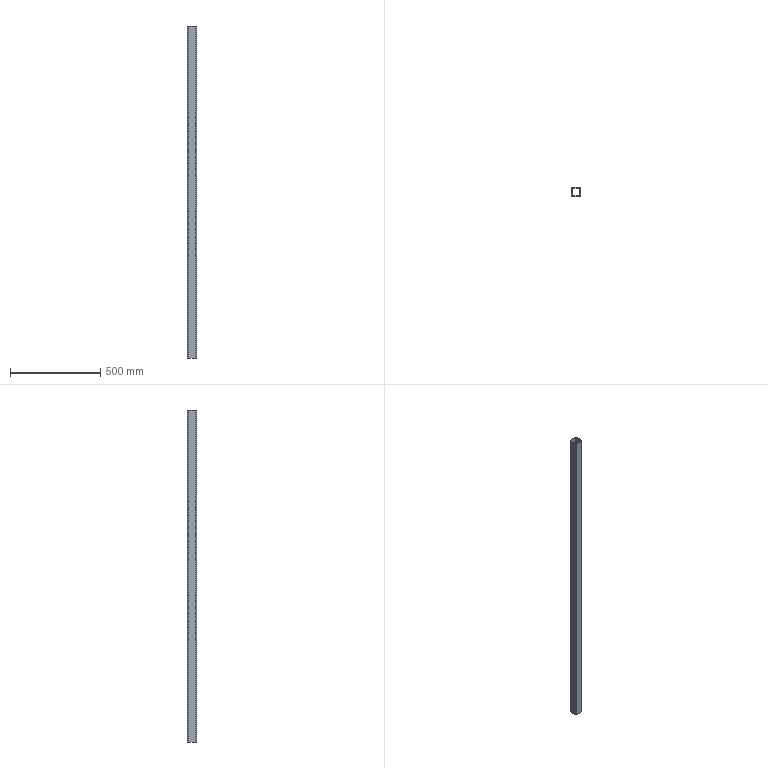Part | SolidWorks | 1 solid | 18 faces | box 50 x 50 x 1840 mm | volume 995114 mm3 | plane 10 | cylinder 8 | commonest cylinder face diameters 6 x4 12 x4
STEP:
#1=CARTESIAN_POINT('',(19.,25.,920.));
#2=VERTEX_POINT('',#1);
#3=CARTESIAN_POINT('',(25.,19.,920.));
#4=VERTEX_POINT('',#3);
#5=CARTESIAN_POINT('',(19.,19.,920.));
#6=DIRECTION('',(0.,0.,-1.));
#7=DIRECTION('',(-1.,0.,0.));
#8=AXIS2_PLACEMENT_3D('',#5,#6,#7);
#9=CIRCLE('',#8,6.);
#10=EDGE_CURVE('',#2,#4,#9,.T.);
#11=ORIENTED_EDGE('',*,*,#10,.T.);
#12=CARTESIAN_POINT('',(25.,19.,-920.));
#13=VERTEX_POINT('',#12);
#14=CARTESIAN_POINT('',(25.,19.,-920.));
#15=DIRECTION('',(0.,0.,1.));
#16=VECTOR('',#15,1000.);
#17=LINE('',#14,#16);
#18=EDGE_CURVE('',#13,#4,#17,.T.);
#19=ORIENTED_EDGE('',*,*,#18,.F.);
#20=CARTESIAN_POINT('',(19.,25.,-920.));
#21=VERTEX_POINT('',#20);
#22=CARTESIAN_POINT('',(19.,19.,-920.));
#23=DIRECTION('',(0.,0.,-1.));
#24=DIRECTION('',(-1.,0.,0.));
#25=AXIS2_PLACEMENT_3D('',#22,#23,#24);
#26=CIRCLE('',#25,6.);
#27=EDGE_CURVE('',#21,#13,#26,.T.);
#28=ORIENTED_EDGE('',*,*,#27,.F.);
#29=CARTESIAN_POINT('',(19.,25.,-920.));
#30=DIRECTION('',(0.,0.,1.));
#31=VECTOR('',#30,1000.);
#32=LINE('',#29,#31);
#33=EDGE_CURVE('',#21,#2,#32,.T.);
#34=ORIENTED_EDGE('',*,*,#33,.T.);
#35=EDGE_LOOP('',(#11,#19,#28,#34));
#36=FACE_OUTER_BOUND('',#35,.T.);
#37=CARTESIAN_POINT('',(19.,19.,-920.));
#38=DIRECTION('',(0.,0.,1.));
#39=DIRECTION('',(1.,0.,0.));
#40=AXIS2_PLACEMENT_3D('',#37,#38,#39);
#41=CYLINDRICAL_SURFACE('',#40,6.);
#42=ADVANCED_FACE('',(#36),#41,.T.);
#43=CARTESIAN_POINT('',(25.,-19.,920.));
#44=VERTEX_POINT('',#43);
#45=CARTESIAN_POINT('',(25.,19.,920.));
#46=DIRECTION('',(0.,-1.,0.));
#47=VECTOR('',#46,1000.);
#48=LINE('',#45,#47);
#49=EDGE_CURVE('',#4,#44,#48,.T.);
#50=ORIENTED_EDGE('',*,*,#49,.T.);
#51=CARTESIAN_POINT('',(25.,-19.,-920.));
#52=VERTEX_POINT('',#51);
#53=CARTESIAN_POINT('',(25.,-19.,-920.));
#54=DIRECTION('',(0.,0.,1.));
#55=VECTOR('',#54,1000.);
#56=LINE('',#53,#55);
#57=EDGE_CURVE('',#52,#44,#56,.T.);
#58=ORIENTED_EDGE('',*,*,#57,.F.);
#59=CARTESIAN_POINT('',(25.,19.,-920.));
#60=DIRECTION('',(0.,-1.,0.));
#61=VECTOR('',#60,1000.);
#62=LINE('',#59,#61);
#63=EDGE_CURVE('',#13,#52,#62,.T.);
#64=ORIENTED_EDGE('',*,*,#63,.F.);
#65=ORIENTED_EDGE('',*,*,#18,.T.);
#66=EDGE_LOOP('',(#50,#58,#64,#65));
#67=FACE_OUTER_BOUND('',#66,.T.);
#68=CARTESIAN_POINT('',(25.,19.,-920.));
#69=DIRECTION('',(-1.,0.,0.));
#70=DIRECTION('',(0.,0.,1.));
#71=AXIS2_PLACEMENT_3D('',#68,#69,#70);
#72=PLANE('',#71);
#73=ADVANCED_FACE('',(#67),#72,.F.);
#74=CARTESIAN_POINT('',(19.,-25.,920.));
#75=VERTEX_POINT('',#74);
#76=CARTESIAN_POINT('',(19.,-19.,920.));
#77=DIRECTION('',(0.,0.,-1.));
#78=DIRECTION('',(-1.,0.,0.));
#79=AXIS2_PLACEMENT_3D('',#76,#77,#78);
#80=CIRCLE('',#79,6.);
#81=EDGE_CURVE('',#44,#75,#80,.T.);
#82=ORIENTED_EDGE('',*,*,#81,.T.);
#83=CARTESIAN_POINT('',(19.,-25.,-920.));
#84=VERTEX_POINT('',#83);
#85=CARTESIAN_POINT('',(19.,-25.,-920.));
#86=DIRECTION('',(0.,0.,1.));
#87=VECTOR('',#86,1000.);
#88=LINE('',#85,#87);
#89=EDGE_CURVE('',#84,#75,#88,.T.);
#90=ORIENTED_EDGE('',*,*,#89,.F.);
#91=CARTESIAN_POINT('',(19.,-19.,-920.));
#92=DIRECTION('',(0.,0.,-1.));
#93=DIRECTION('',(-1.,0.,0.));
#94=AXIS2_PLACEMENT_3D('',#91,#92,#93);
#95=CIRCLE('',#94,6.);
#96=EDGE_CURVE('',#52,#84,#95,.T.);
#97=ORIENTED_EDGE('',*,*,#96,.F.);
#98=ORIENTED_EDGE('',*,*,#57,.T.);
#99=EDGE_LOOP('',(#82,#90,#97,#98));
#100=FACE_OUTER_BOUND('',#99,.T.);
#101=CARTESIAN_POINT('',(19.,-19.,-920.));
#102=DIRECTION('',(0.,0.,1.));
#103=DIRECTION('',(1.,0.,0.));
#104=AXIS2_PLACEMENT_3D('',#101,#102,#103);
#105=CYLINDRICAL_SURFACE('',#104,6.);
#106=ADVANCED_FACE('',(#100),#105,.T.);
#107=CARTESIAN_POINT('',(-19.,-25.,920.));
#108=VERTEX_POINT('',#107);
#109=CARTESIAN_POINT('',(-19.,-25.,920.));
#110=DIRECTION('',(-1.,0.,0.));
#111=VECTOR('',#110,1000.);
#112=LINE('',#109,#111);
#113=EDGE_CURVE('',#75,#108,#112,.T.);
#114=ORIENTED_EDGE('',*,*,#113,.T.);
#115=CARTESIAN_POINT('',(-19.,-25.,-920.));
#116=VERTEX_POINT('',#115);
#117=CARTESIAN_POINT('',(-19.,-25.,-920.));
#118=DIRECTION('',(0.,0.,1.));
#119=VECTOR('',#118,1000.);
#120=LINE('',#117,#119);
#121=EDGE_CURVE('',#116,#108,#120,.T.);
#122=ORIENTED_EDGE('',*,*,#121,.F.);
#123=CARTESIAN_POINT('',(-19.,-25.,-920.));
#124=DIRECTION('',(-1.,0.,0.));
#125=VECTOR('',#124,1000.);
#126=LINE('',#123,#125);
#127=EDGE_CURVE('',#84,#116,#126,.T.);
#128=ORIENTED_EDGE('',*,*,#127,.F.);
#129=ORIENTED_EDGE('',*,*,#89,.T.);
#130=EDGE_LOOP('',(#114,#122,#128,#129));
#131=FACE_OUTER_BOUND('',#130,.T.);
#132=CARTESIAN_POINT('',(-19.,-25.,-920.));
#133=DIRECTION('',(0.,1.,0.));
#134=DIRECTION('',(0.,0.,1.));
#135=AXIS2_PLACEMENT_3D('',#132,#133,#134);
#136=PLANE('',#135);
#137=ADVANCED_FACE('',(#131),#136,.F.);
#138=CARTESIAN_POINT('',(-25.,-19.,920.));
#139=VERTEX_POINT('',#138);
#140=CARTESIAN_POINT('',(-19.,-19.,920.));
#141=DIRECTION('',(0.,0.,-1.));
#142=DIRECTION('',(-1.,0.,0.));
#143=AXIS2_PLACEMENT_3D('',#140,#141,#142);
#144=CIRCLE('',#143,6.);
#145=EDGE_CURVE('',#108,#139,#144,.T.);
#146=ORIENTED_EDGE('',*,*,#145,.T.);
#147=CARTESIAN_POINT('',(-25.,-19.,-920.));
#148=VERTEX_POINT('',#147);
#149=CARTESIAN_POINT('',(-25.,-19.,-920.));
#150=DIRECTION('',(0.,0.,1.));
#151=VECTOR('',#150,1000.);
#152=LINE('',#149,#151);
#153=EDGE_CURVE('',#148,#139,#152,.T.);
#154=ORIENTED_EDGE('',*,*,#153,.F.);
#155=CARTESIAN_POINT('',(-19.,-19.,-920.));
#156=DIRECTION('',(0.,0.,-1.));
#157=DIRECTION('',(-1.,0.,0.));
#158=AXIS2_PLACEMENT_3D('',#155,#156,#157);
#159=CIRCLE('',#158,6.);
#160=EDGE_CURVE('',#116,#148,#159,.T.);
#161=ORIENTED_EDGE('',*,*,#160,.F.);
#162=ORIENTED_EDGE('',*,*,#121,.T.);
#163=EDGE_LOOP('',(#146,#154,#161,#162));
#164=FACE_OUTER_BOUND('',#163,.T.);
#165=CARTESIAN_POINT('',(-19.,-19.,-920.));
#166=DIRECTION('',(0.,0.,1.));
#167=DIRECTION('',(1.,0.,0.));
#168=AXIS2_PLACEMENT_3D('',#165,#166,#167);
#169=CYLINDRICAL_SURFACE('',#168,6.);
#170=ADVANCED_FACE('',(#164),#169,.T.);
#171=CARTESIAN_POINT('',(-25.,19.,920.));
#172=VERTEX_POINT('',#171);
#173=CARTESIAN_POINT('',(-25.,-19.,920.));
#174=DIRECTION('',(0.,1.,0.));
#175=VECTOR('',#174,1000.);
#176=LINE('',#173,#175);
#177=EDGE_CURVE('',#139,#172,#176,.T.);
#178=ORIENTED_EDGE('',*,*,#177,.T.);
#179=CARTESIAN_POINT('',(-25.,19.,-920.));
#180=VERTEX_POINT('',#179);
#181=CARTESIAN_POINT('',(-25.,19.,-920.));
#182=DIRECTION('',(0.,0.,1.));
#183=VECTOR('',#182,1000.);
#184=LINE('',#181,#183);
#185=EDGE_CURVE('',#180,#172,#184,.T.);
#186=ORIENTED_EDGE('',*,*,#185,.F.);
#187=CARTESIAN_POINT('',(-25.,-19.,-920.));
#188=DIRECTION('',(0.,1.,0.));
#189=VECTOR('',#188,1000.);
#190=LINE('',#187,#189);
#191=EDGE_CURVE('',#148,#180,#190,.T.);
#192=ORIENTED_EDGE('',*,*,#191,.F.);
#193=ORIENTED_EDGE('',*,*,#153,.T.);
#194=EDGE_LOOP('',(#178,#186,#192,#193));
#195=FACE_OUTER_BOUND('',#194,.T.);
#196=CARTESIAN_POINT('',(-25.,-19.,-920.));
#197=DIRECTION('',(1.,0.,0.));
#198=DIRECTION('',(0.,0.,-1.));
#199=AXIS2_PLACEMENT_3D('',#196,#197,#198);
#200=PLANE('',#199);
#201=ADVANCED_FACE('',(#195),#200,.F.);
#202=CARTESIAN_POINT('',(-19.,25.,920.));
#203=VERTEX_POINT('',#202);
#204=CARTESIAN_POINT('',(-19.,19.,920.));
#205=DIRECTION('',(0.,0.,-1.));
#206=DIRECTION('',(-1.,0.,0.));
#207=AXIS2_PLACEMENT_3D('',#204,#205,#206);
#208=CIRCLE('',#207,6.);
#209=EDGE_CURVE('',#172,#203,#208,.T.);
#210=ORIENTED_EDGE('',*,*,#209,.T.);
#211=CARTESIAN_POINT('',(-19.,25.,-920.));
#212=VERTEX_POINT('',#211);
#213=CARTESIAN_POINT('',(-19.,25.,-920.));
#214=DIRECTION('',(0.,0.,1.));
#215=VECTOR('',#214,1000.);
#216=LINE('',#213,#215);
#217=EDGE_CURVE('',#212,#203,#216,.T.);
#218=ORIENTED_EDGE('',*,*,#217,.F.);
#219=CARTESIAN_POINT('',(-19.,19.,-920.));
#220=DIRECTION('',(0.,0.,-1.));
#221=DIRECTION('',(-1.,0.,0.));
#222=AXIS2_PLACEMENT_3D('',#219,#220,#221);
#223=CIRCLE('',#222,6.);
#224=EDGE_CURVE('',#180,#212,#223,.T.);
#225=ORIENTED_EDGE('',*,*,#224,.F.);
#226=ORIENTED_EDGE('',*,*,#185,.T.);
#227=EDGE_LOOP('',(#210,#218,#225,#226));
#228=FACE_OUTER_BOUND('',#227,.T.);
#229=CARTESIAN_POINT('',(-19.,19.,-920.));
#230=DIRECTION('',(0.,0.,1.));
#231=DIRECTION('',(1.,0.,0.));
#232=AXIS2_PLACEMENT_3D('',#229,#230,#231);
#233=CYLINDRICAL_SURFACE('',#232,6.);
#234=ADVANCED_FACE('',(#228),#233,.T.);
#235=CARTESIAN_POINT('',(22.,-19.,920.));
#236=VERTEX_POINT('',#235);
#237=CARTESIAN_POINT('',(19.,-22.,920.));
#238=VERTEX_POINT('',#237);
#239=CARTESIAN_POINT('',(19.,-19.,920.));
#240=DIRECTION('',(0.,0.,-1.));
#241=DIRECTION('',(-1.,0.,0.));
#242=AXIS2_PLACEMENT_3D('',#239,#240,#241);
#243=CIRCLE('',#242,3.);
#244=EDGE_CURVE('',#236,#238,#243,.T.);
#245=ORIENTED_EDGE('',*,*,#244,.F.);
#246=CARTESIAN_POINT('',(22.,-19.,-920.));
#247=VERTEX_POINT('',#246);
#248=CARTESIAN_POINT('',(22.,-19.,-920.));
#249=DIRECTION('',(0.,0.,1.));
#250=VECTOR('',#249,1000.);
#251=LINE('',#248,#250);
#252=EDGE_CURVE('',#247,#236,#251,.T.);
#253=ORIENTED_EDGE('',*,*,#252,.F.);
#254=CARTESIAN_POINT('',(19.,-22.,-920.));
#255=VERTEX_POINT('',#254);
#256=CARTESIAN_POINT('',(19.,-19.,-920.));
#257=DIRECTION('',(0.,0.,-1.));
#258=DIRECTION('',(-1.,0.,0.));
#259=AXIS2_PLACEMENT_3D('',#256,#257,#258);
#260=CIRCLE('',#259,3.);
#261=EDGE_CURVE('',#247,#255,#260,.T.);
#262=ORIENTED_EDGE('',*,*,#261,.T.);
#263=CARTESIAN_POINT('',(19.,-22.,-920.));
#264=DIRECTION('',(0.,0.,1.));
#265=VECTOR('',#264,1000.);
#266=LINE('',#263,#265);
#267=EDGE_CURVE('',#255,#238,#266,.T.);
#268=ORIENTED_EDGE('',*,*,#267,.T.);
#269=EDGE_LOOP('',(#245,#253,#262,#268));
#270=FACE_OUTER_BOUND('',#269,.T.);
#271=CARTESIAN_POINT('',(19.,-19.,-920.));
#272=DIRECTION('',(0.,0.,1.));
#273=DIRECTION('',(1.,0.,0.));
#274=AXIS2_PLACEMENT_3D('',#271,#272,#273);
#275=CYLINDRICAL_SURFACE('',#274,3.);
#276=ADVANCED_FACE('',(#270),#275,.F.);
#277=CARTESIAN_POINT('',(22.,19.,920.));
#278=VERTEX_POINT('',#277);
#279=CARTESIAN_POINT('',(22.,19.,920.));
#280=DIRECTION('',(0.,-1.,0.));
#281=VECTOR('',#280,1000.);
#282=LINE('',#279,#281);
#283=EDGE_CURVE('',#278,#236,#282,.T.);
#284=ORIENTED_EDGE('',*,*,#283,.F.);
#285=CARTESIAN_POINT('',(22.,19.,-920.));
#286=VERTEX_POINT('',#285);
#287=CARTESIAN_POINT('',(22.,19.,-920.));
#288=DIRECTION('',(0.,0.,1.));
#289=VECTOR('',#288,1000.);
#290=LINE('',#287,#289);
#291=EDGE_CURVE('',#286,#278,#290,.T.);
#292=ORIENTED_EDGE('',*,*,#291,.F.);
#293=CARTESIAN_POINT('',(22.,19.,-920.));
#294=DIRECTION('',(0.,-1.,0.));
#295=VECTOR('',#294,1000.);
#296=LINE('',#293,#295);
#297=EDGE_CURVE('',#286,#247,#296,.T.);
#298=ORIENTED_EDGE('',*,*,#297,.T.);
#299=ORIENTED_EDGE('',*,*,#252,.T.);
#300=EDGE_LOOP('',(#284,#292,#298,#299));
#301=FACE_OUTER_BOUND('',#300,.T.);
#302=CARTESIAN_POINT('',(22.,19.,-920.));
#303=DIRECTION('',(-1.,0.,0.));
#304=DIRECTION('',(0.,0.,1.));
#305=AXIS2_PLACEMENT_3D('',#302,#303,#304);
#306=PLANE('',#305);
#307=ADVANCED_FACE('',(#301),#306,.T.);
#308=CARTESIAN_POINT('',(19.,22.,920.));
#309=VERTEX_POINT('',#308);
#310=CARTESIAN_POINT('',(19.,19.,920.));
#311=DIRECTION('',(0.,0.,-1.));
#312=DIRECTION('',(-1.,0.,0.));
#313=AXIS2_PLACEMENT_3D('',#310,#311,#312);
#314=CIRCLE('',#313,3.);
#315=EDGE_CURVE('',#309,#278,#314,.T.);
#316=ORIENTED_EDGE('',*,*,#315,.F.);
#317=CARTESIAN_POINT('',(19.,22.,-920.));
#318=VERTEX_POINT('',#317);
#319=CARTESIAN_POINT('',(19.,22.,-920.));
#320=DIRECTION('',(0.,0.,1.));
#321=VECTOR('',#320,1000.);
#322=LINE('',#319,#321);
#323=EDGE_CURVE('',#318,#309,#322,.T.);
#324=ORIENTED_EDGE('',*,*,#323,.F.);
#325=CARTESIAN_POINT('',(19.,19.,-920.));
#326=DIRECTION('',(0.,0.,-1.));
#327=DIRECTION('',(-1.,0.,0.));
#328=AXIS2_PLACEMENT_3D('',#325,#326,#327);
#329=CIRCLE('',#328,3.);
#330=EDGE_CURVE('',#318,#286,#329,.T.);
#331=ORIENTED_EDGE('',*,*,#330,.T.);
#332=ORIENTED_EDGE('',*,*,#291,.T.);
#333=EDGE_LOOP('',(#316,#324,#331,#332));
#334=FACE_OUTER_BOUND('',#333,.T.);
#335=CARTESIAN_POINT('',(19.,19.,-920.));
#336=DIRECTION('',(0.,0.,1.));
#337=DIRECTION('',(1.,0.,0.));
#338=AXIS2_PLACEMENT_3D('',#335,#336,#337);
#339=CYLINDRICAL_SURFACE('',#338,3.);
#340=ADVANCED_FACE('',(#334),#339,.F.);
#341=CARTESIAN_POINT('',(-19.,22.,920.));
#342=VERTEX_POINT('',#341);
#343=CARTESIAN_POINT('',(19.,22.,920.));
#344=DIRECTION('',(1.,0.,0.));
#345=VECTOR('',#344,1000.);
#346=LINE('',#343,#345);
#347=EDGE_CURVE('',#342,#309,#346,.T.);
#348=ORIENTED_EDGE('',*,*,#347,.F.);
#349=CARTESIAN_POINT('',(-19.,22.,-920.));
#350=VERTEX_POINT('',#349);
#351=CARTESIAN_POINT('',(-19.,22.,-920.));
#352=DIRECTION('',(0.,0.,1.));
#353=VECTOR('',#352,1000.);
#354=LINE('',#351,#353);
#355=EDGE_CURVE('',#350,#342,#354,.T.);
#356=ORIENTED_EDGE('',*,*,#355,.F.);
#357=CARTESIAN_POINT('',(19.,22.,-920.));
#358=DIRECTION('',(1.,0.,0.));
#359=VECTOR('',#358,1000.);
#360=LINE('',#357,#359);
#361=EDGE_CURVE('',#350,#318,#360,.T.);
#362=ORIENTED_EDGE('',*,*,#361,.T.);
#363=ORIENTED_EDGE('',*,*,#323,.T.);
#364=EDGE_LOOP('',(#348,#356,#362,#363));
#365=FACE_OUTER_BOUND('',#364,.T.);
#366=CARTESIAN_POINT('',(19.,22.,-920.));
#367=DIRECTION('',(0.,-1.,0.));
#368=DIRECTION('',(0.,0.,-1.));
#369=AXIS2_PLACEMENT_3D('',#366,#367,#368);
#370=PLANE('',#369);
#371=ADVANCED_FACE('',(#365),#370,.T.);
#372=CARTESIAN_POINT('',(-22.,19.,920.));
#373=VERTEX_POINT('',#372);
#374=CARTESIAN_POINT('',(-19.,19.,920.));
#375=DIRECTION('',(0.,0.,-1.));
#376=DIRECTION('',(-1.,0.,0.));
#377=AXIS2_PLACEMENT_3D('',#374,#375,#376);
#378=CIRCLE('',#377,3.);
#379=EDGE_CURVE('',#373,#342,#378,.T.);
#380=ORIENTED_EDGE('',*,*,#379,.F.);
#381=CARTESIAN_POINT('',(-22.,19.,-920.));
#382=VERTEX_POINT('',#381);
#383=CARTESIAN_POINT('',(-22.,19.,-920.));
#384=DIRECTION('',(0.,0.,1.));
#385=VECTOR('',#384,1000.);
#386=LINE('',#383,#385);
#387=EDGE_CURVE('',#382,#373,#386,.T.);
#388=ORIENTED_EDGE('',*,*,#387,.F.);
#389=CARTESIAN_POINT('',(-19.,19.,-920.));
#390=DIRECTION('',(0.,0.,-1.));
#391=DIRECTION('',(-1.,0.,0.));
#392=AXIS2_PLACEMENT_3D('',#389,#390,#391);
#393=CIRCLE('',#392,3.);
#394=EDGE_CURVE('',#382,#350,#393,.T.);
#395=ORIENTED_EDGE('',*,*,#394,.T.);
#396=ORIENTED_EDGE('',*,*,#355,.T.);
#397=EDGE_LOOP('',(#380,#388,#395,#396));
#398=FACE_OUTER_BOUND('',#397,.T.);
#399=CARTESIAN_POINT('',(-19.,19.,-920.));
#400=DIRECTION('',(0.,0.,1.));
#401=DIRECTION('',(1.,0.,0.));
#402=AXIS2_PLACEMENT_3D('',#399,#400,#401);
#403=CYLINDRICAL_SURFACE('',#402,3.);
#404=ADVANCED_FACE('',(#398),#403,.F.);
#405=CARTESIAN_POINT('',(-22.,-19.,920.));
#406=VERTEX_POINT('',#405);
#407=CARTESIAN_POINT('',(-22.,-19.,920.));
#408=DIRECTION('',(0.,1.,0.));
#409=VECTOR('',#408,1000.);
#410=LINE('',#407,#409);
#411=EDGE_CURVE('',#406,#373,#410,.T.);
#412=ORIENTED_EDGE('',*,*,#411,.F.);
#413=CARTESIAN_POINT('',(-22.,-19.,-920.));
#414=VERTEX_POINT('',#413);
#415=CARTESIAN_POINT('',(-22.,-19.,-920.));
#416=DIRECTION('',(0.,0.,1.));
#417=VECTOR('',#416,1000.);
#418=LINE('',#415,#417);
#419=EDGE_CURVE('',#414,#406,#418,.T.);
#420=ORIENTED_EDGE('',*,*,#419,.F.);
#421=CARTESIAN_POINT('',(-22.,-19.,-920.));
#422=DIRECTION('',(0.,1.,0.));
#423=VECTOR('',#422,1000.);
#424=LINE('',#421,#423);
#425=EDGE_CURVE('',#414,#382,#424,.T.);
#426=ORIENTED_EDGE('',*,*,#425,.T.);
#427=ORIENTED_EDGE('',*,*,#387,.T.);
#428=EDGE_LOOP('',(#412,#420,#426,#427));
#429=FACE_OUTER_BOUND('',#428,.T.);
#430=CARTESIAN_POINT('',(-22.,-19.,-920.));
#431=DIRECTION('',(1.,0.,0.));
#432=DIRECTION('',(0.,0.,-1.));
#433=AXIS2_PLACEMENT_3D('',#430,#431,#432);
#434=PLANE('',#433);
#435=ADVANCED_FACE('',(#429),#434,.T.);
#436=CARTESIAN_POINT('',(-19.,-22.,920.));
#437=VERTEX_POINT('',#436);
#438=CARTESIAN_POINT('',(-19.,-19.,920.));
#439=DIRECTION('',(0.,0.,-1.));
#440=DIRECTION('',(-1.,0.,0.));
#441=AXIS2_PLACEMENT_3D('',#438,#439,#440);
#442=CIRCLE('',#441,3.);
#443=EDGE_CURVE('',#437,#406,#442,.T.);
#444=ORIENTED_EDGE('',*,*,#443,.F.);
#445=CARTESIAN_POINT('',(-19.,-22.,-920.));
#446=VERTEX_POINT('',#445);
#447=CARTESIAN_POINT('',(-19.,-22.,-920.));
#448=DIRECTION('',(0.,0.,1.));
#449=VECTOR('',#448,1000.);
#450=LINE('',#447,#449);
#451=EDGE_CURVE('',#446,#437,#450,.T.);
#452=ORIENTED_EDGE('',*,*,#451,.F.);
#453=CARTESIAN_POINT('',(-19.,-19.,-920.));
#454=DIRECTION('',(0.,0.,-1.));
#455=DIRECTION('',(-1.,0.,0.));
#456=AXIS2_PLACEMENT_3D('',#453,#454,#455);
#457=CIRCLE('',#456,3.);
#458=EDGE_CURVE('',#446,#414,#457,.T.);
#459=ORIENTED_EDGE('',*,*,#458,.T.);
#460=ORIENTED_EDGE('',*,*,#419,.T.);
#461=EDGE_LOOP('',(#444,#452,#459,#460));
#462=FACE_OUTER_BOUND('',#461,.T.);
#463=CARTESIAN_POINT('',(-19.,-19.,-920.));
#464=DIRECTION('',(0.,0.,1.));
#465=DIRECTION('',(1.,0.,0.));
#466=AXIS2_PLACEMENT_3D('',#463,#464,#465);
#467=CYLINDRICAL_SURFACE('',#466,3.);
#468=ADVANCED_FACE('',(#462),#467,.F.);
#469=CARTESIAN_POINT('',(-19.,-22.,920.));
#470=DIRECTION('',(-1.,0.,0.));
#471=VECTOR('',#470,1000.);
#472=LINE('',#469,#471);
#473=EDGE_CURVE('',#238,#437,#472,.T.);
#474=ORIENTED_EDGE('',*,*,#473,.F.);
#475=ORIENTED_EDGE('',*,*,#267,.F.);
#476=CARTESIAN_POINT('',(-19.,-22.,-920.));
#477=DIRECTION('',(-1.,0.,0.));
#478=VECTOR('',#477,1000.);
#479=LINE('',#476,#478);
#480=EDGE_CURVE('',#255,#446,#479,.T.);
#481=ORIENTED_EDGE('',*,*,#480,.T.);
#482=ORIENTED_EDGE('',*,*,#451,.T.);
#483=EDGE_LOOP('',(#474,#475,#481,#482));
#484=FACE_OUTER_BOUND('',#483,.T.);
#485=CARTESIAN_POINT('',(-19.,-22.,-920.));
#486=DIRECTION('',(0.,1.,0.));
#487=DIRECTION('',(0.,0.,1.));
#488=AXIS2_PLACEMENT_3D('',#485,#486,#487);
#489=PLANE('',#488);
#490=ADVANCED_FACE('',(#484),#489,.T.);
#491=CARTESIAN_POINT('',(19.,25.,920.));
#492=DIRECTION('',(1.,0.,0.));
#493=VECTOR('',#492,1000.);
#494=LINE('',#491,#493);
#495=EDGE_CURVE('',#203,#2,#494,.T.);
#496=ORIENTED_EDGE('',*,*,#495,.T.);
#497=ORIENTED_EDGE('',*,*,#33,.F.);
#498=CARTESIAN_POINT('',(19.,25.,-920.));
#499=DIRECTION('',(1.,0.,0.));
#500=VECTOR('',#499,1000.);
#501=LINE('',#498,#500);
#502=EDGE_CURVE('',#212,#21,#501,.T.);
#503=ORIENTED_EDGE('',*,*,#502,.F.);
#504=ORIENTED_EDGE('',*,*,#217,.T.);
#505=EDGE_LOOP('',(#496,#497,#503,#504));
#506=FACE_OUTER_BOUND('',#505,.T.);
#507=CARTESIAN_POINT('',(19.,25.,-920.));
#508=DIRECTION('',(0.,-1.,0.));
#509=DIRECTION('',(0.,0.,-1.));
#510=AXIS2_PLACEMENT_3D('',#507,#508,#509);
#511=PLANE('',#510);
#512=ADVANCED_FACE('',(#506),#511,.F.);
#513=ORIENTED_EDGE('',*,*,#261,.F.);
#514=ORIENTED_EDGE('',*,*,#297,.F.);
#515=ORIENTED_EDGE('',*,*,#330,.F.);
#516=ORIENTED_EDGE('',*,*,#361,.F.);
#517=ORIENTED_EDGE('',*,*,#394,.F.);
#518=ORIENTED_EDGE('',*,*,#425,.F.);
#519=ORIENTED_EDGE('',*,*,#458,.F.);
#520=ORIENTED_EDGE('',*,*,#480,.F.);
#521=EDGE_LOOP('',(#513,#514,#515,#516,#517,#518,#519,#520));
#522=FACE_BOUND('',#521,.T.);
#523=ORIENTED_EDGE('',*,*,#27,.T.);
#524=ORIENTED_EDGE('',*,*,#63,.T.);
#525=ORIENTED_EDGE('',*,*,#96,.T.);
#526=ORIENTED_EDGE('',*,*,#127,.T.);
#527=ORIENTED_EDGE('',*,*,#160,.T.);
#528=ORIENTED_EDGE('',*,*,#191,.T.);
#529=ORIENTED_EDGE('',*,*,#224,.T.);
#530=ORIENTED_EDGE('',*,*,#502,.T.);
#531=EDGE_LOOP('',(#523,#524,#525,#526,#527,#528,#529,#530));
#532=FACE_OUTER_BOUND('',#531,.T.);
#533=CARTESIAN_POINT('',(19.,19.,-920.));
#534=DIRECTION('',(0.,0.,-1.));
#535=DIRECTION('',(-1.,0.,0.));
#536=AXIS2_PLACEMENT_3D('',#533,#534,#535);
#537=PLANE('',#536);
#538=ADVANCED_FACE('',(#522,#532),#537,.T.);
#539=ORIENTED_EDGE('',*,*,#244,.T.);
#540=ORIENTED_EDGE('',*,*,#473,.T.);
#541=ORIENTED_EDGE('',*,*,#443,.T.);
#542=ORIENTED_EDGE('',*,*,#411,.T.);
#543=ORIENTED_EDGE('',*,*,#379,.T.);
#544=ORIENTED_EDGE('',*,*,#347,.T.);
#545=ORIENTED_EDGE('',*,*,#315,.T.);
#546=ORIENTED_EDGE('',*,*,#283,.T.);
#547=EDGE_LOOP('',(#539,#540,#541,#542,#543,#544,#545,#546));
#548=FACE_BOUND('',#547,.T.);
#549=ORIENTED_EDGE('',*,*,#10,.F.);
#550=ORIENTED_EDGE('',*,*,#495,.F.);
#551=ORIENTED_EDGE('',*,*,#209,.F.);
#552=ORIENTED_EDGE('',*,*,#177,.F.);
#553=ORIENTED_EDGE('',*,*,#145,.F.);
#554=ORIENTED_EDGE('',*,*,#113,.F.);
#555=ORIENTED_EDGE('',*,*,#81,.F.);
#556=ORIENTED_EDGE('',*,*,#49,.F.);
#557=EDGE_LOOP('',(#549,#550,#551,#552,#553,#554,#555,#556));
#558=FACE_OUTER_BOUND('',#557,.T.);
#559=CARTESIAN_POINT('',(19.,19.,920.));
#560=DIRECTION('',(0.,0.,-1.));
#561=DIRECTION('',(-1.,0.,0.));
#562=AXIS2_PLACEMENT_3D('',#559,#560,#561);
#563=PLANE('',#562);
#564=ADVANCED_FACE('',(#548,#558),#563,.F.);
#565=CLOSED_SHELL('',(#42,#73,#106,#137,#170,#201,#234,#276,#307,#340,#371,#404,#435,#468,#490,#512,#538,#564));
#566=MANIFOLD_SOLID_BREP('',#565);
#567=CARTESIAN_POINT('',(0.,0.,0.));
#568=DIRECTION('',(0.,0.,1.));
#569=DIRECTION('',(1.,0.,0.));
#570=AXIS2_PLACEMENT_3D('',#567,#568,#569);
#571=(LENGTH_UNIT()NAMED_UNIT(*)SI_UNIT(.MILLI.,.METRE.));
#572=UNCERTAINTY_MEASURE_WITH_UNIT(LENGTH_MEASURE(0.00001),#571,'','');
#573=(NAMED_UNIT(*)PLANE_ANGLE_UNIT()SI_UNIT($,.RADIAN.));
#574=(NAMED_UNIT(*)SI_UNIT($,.STERADIAN.)SOLID_ANGLE_UNIT());
#575=(GEOMETRIC_REPRESENTATION_CONTEXT(3)GLOBAL_UNCERTAINTY_ASSIGNED_CONTEXT((#572))GLOBAL_UNIT_ASSIGNED_CONTEXT((#571,#573,#574))REPRESENTATION_CONTEXT('',''));
#576=ADVANCED_BREP_SHAPE_REPRESENTATION('',(#566,#570),#575);